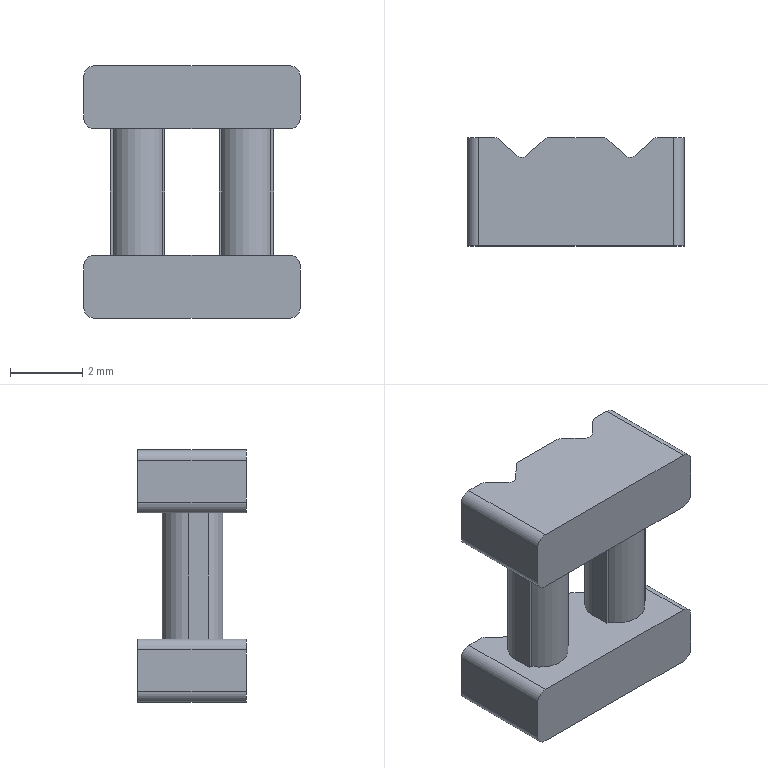Part | SolidWorks | features Fillet 8, ICE 3, Extrusion 1 | 1 solid | 56 faces | box 6 x 3 x 7 mm | volume 74.604 mm3 | plane 32 | cylinder 24 | commonest cylinder face diameters 0.4 x12 0.6 x8 1.52 x4